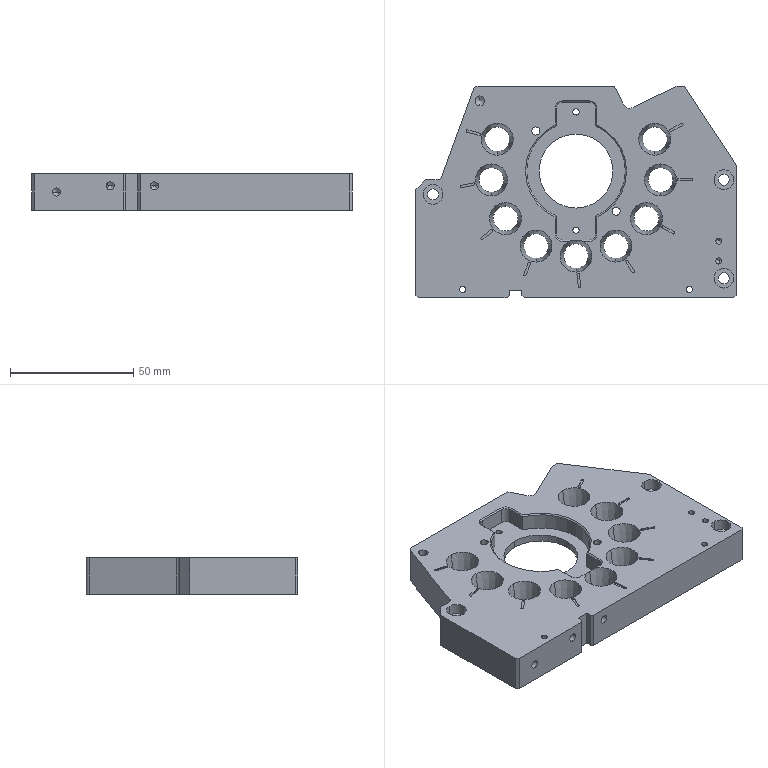NC program | NX | posted with a generic post | part box 130 x 86 x 15 mm
Whole program:
N10 G17 G21 G94 G90
(DRILLING_COPY_2 , TOOL : ZXZ)
N12 T21 M6
N14 G54
N16 G17 G0 G90 X15.25 Y-2.5 B0. C0. S3500 M3
N18 G43 Z30. H21
N20 G94 G81 G98 Z-1. F250. R3.
N22 X55. Y0.
N24 X33.25 Y-2.5
N26 G80
N28 G0 X33.25 Y-2.5 Z30.
N30 M5
(DRILLING_COPY_1_COPY_1 , TOOL : 3.3ZT)
N32 T13 M6
N34 G54
N36 G17 G0 G90 X15.25 Y-2.5 B0. C0. S2000 M3
N38 G43 Z30. H13
N40 G94 G83 G98 Z-11.091 F150. Q2. R3.
N42 X55. Y0. Z-5.991
N44 X33.25 Y-2.5 Z-11.091
N46 G80
N48 G0 X33.25 Y-2.5 Z30.
N50 M5
(ZLEVEL_PROFILE_1_COPY_COPY_1 , TOOL : D4)
N52 T17 M6
N54 G54
N56 G17 G0 G90 X24.698 Y13.381 B0. C0. S7500 M3
N58 G43 Z30. H17
N60 Z0.5
N62 G94 G1 X24.689 Y13.375 Z0.403 F1000.
N64 X24.664 Y13.354 Z0.316
N66 X24.627 Y13.318 Z0.239
N68 X24.579 Y13.264 Z0.171
N70 X24.523 Y13.192 Z0.113
N72 X24.462 Y13.098 Z0.062
N74 X24.398 Y12.981 Z0.02
N76 X24.334 Y12.84 Z-0.015
N78 X24.273 Y12.673 Z-0.043
N80 X24.217 Y12.477 Z-0.065
N82 X24.169 Y12.252 Z-0.081
N84 X24.131 Y11.996 Z-0.092
N86 X24.107 Y11.706 Z-0.098
N88 X24.098 Y11.381 Z-0.1
N90 X24.1 Y6.871 F1650.
N92 Y-7.493
N94 X24.098 Y-11.381
N96 X24.106 Y-11.461
N98 X24.127 Y-11.53
N100 X24.158 Y-11.588
N102 X24.198 Y-11.637
N104 X24.244 Y-11.676
N106 X24.292 Y-11.708
N108 X24.341 Y-11.733
N110 X24.422 Y-11.761
N112 X24.5 Y-11.77
N114 X24.578 Y-11.761
N116 X24.659 Y-11.733
N118 X24.708 Y-11.708
N120 X24.756 Y-11.676
N122 X24.802 Y-11.637
N124 X24.842 Y-11.588
N126 X24.873 Y-11.53
N128 X24.894 Y-11.461
N130 X24.902 Y-11.381
N132 Y-7.503
N134 X24.9 Y-7.485
N136 Y6.871
N138 X24.902 Y11.381
N140 X24.894 Y11.462 Z-0.101
N142 X24.873 Y11.531 Z-0.103
N144 X24.842 Y11.59 Z-0.106
N146 X24.802 Y11.639 Z-0.11
N148 X24.756 Y11.679 Z-0.115
N150 X24.708 Y11.711 Z-0.121
N152 X24.659 Y11.736 Z-0.127
N154 X24.578 Y11.765 Z-0.138
N156 X24.5 Y11.775 Z-0.15
N158 X24.422 Y11.766 Z-0.162
N160 X24.341 Y11.738 Z-0.173
N162 X24.292 Y11.714 Z-0.179
N164 X24.244 Y11.682 Z-0.185
N166 X24.198 Y11.642 Z-0.19
N168 X24.158 Y11.593 Z-0.194
N170 X24.127 Y11.535 Z-0.197
N172 X24.106 Y11.466 Z-0.199
N174 X24.098 Y11.385 Z-0.2
N176 X24.1 Y6.871
N178 Y-7.493
N180 X24.098 Y-11.385
N182 X24.106 Y-11.465
N184 X24.127 Y-11.534
N186 X24.158 Y-11.592
N188 X24.198 Y-11.641
N190 X24.244 Y-11.68
N192 X24.292 Y-11.712
N194 X24.341 Y-11.737
N196 X24.422 Y-11.765
N198 X24.5 Y-11.774
N200 X24.578 Y-11.765
N202 X24.659 Y-11.737
N204 X24.708 Y-11.712
N206 X24.756 Y-11.68
N208 X24.802 Y-11.641
N210 X24.842 Y-11.592
N212 X24.873 Y-11.534
N214 X24.894 Y-11.465
N216 X24.902 Y-11.385
N218 Y-7.503
N220 X24.9 Y-7.485
N222 Y6.871
N224 X24.902 Y11.385
N226 X24.894 Y11.466 Z-0.201
N228 X24.873 Y11.535 Z-0.203
N230 X24.842 Y11.594 Z-0.206
N232 X24.802 Y11.643 Z-0.21
N234 X24.756 Y11.683 Z-0.215
N236 X24.708 Y11.715 Z-0.221
N238 X24.659 Y11.74 Z-0.227
N240 X24.578 Y11.769 Z-0.238
N242 X24.5 Y11.779 Z-0.25
N244 X24.422 Y11.77 Z-0.262
N246 X24.341 Y11.742 Z-0.273
N248 X24.292 Y11.718 Z-0.279
N250 X24.244 Y11.686 Z-0.285
N252 X24.198 Y11.646 Z-0.29
N254 X24.159 Y11.597 Z-0.294
N256 X24.127 Y11.539 Z-0.297
N258 X24.106 Y11.47 Z-0.299
N260 X24.098 Y11.389 Z-0.3
N262 X24.1 Y6.871
N264 Y-7.493
N266 X24.098 Y-11.389
N268 X24.106 Y-11.469
N270 X24.127 Y-11.538
N272 X24.158 Y-11.596
N274 X24.198 Y-11.645
N276 X24.244 Y-11.684
N278 X24.292 Y-11.716
N280 X24.341 Y-11.741
N282 X24.422 Y-11.769
N284 X24.5 Y-11.778
N286 X24.578 Y-11.769
N288 X24.659 Y-11.741
N290 X24.708 Y-11.716
N292 X24.756 Y-11.684
N294 X24.802 Y-11.645
N296 X24.842 Y-11.596
N298 X24.873 Y-11.538
N300 X24.894 Y-11.469
N302 X24.902 Y-11.389
N304 Y-7.503
N306 X24.9 Y-7.485
N308 Y6.871
N310 X24.902 Y11.389
N312 X24.894 Y11.47 Z-0.301
N314 X24.873 Y11.539 Z-0.303
N316 X24.841 Y11.598 Z-0.306
N318 X24.802 Y11.647 Z-0.31
N320 X24.756 Y11.687 Z-0.315
N322 X24.708 Y11.719 Z-0.321
N324 X24.659 Y11.745 Z-0.327
N326 X24.578 Y11.773 Z-0.338
N328 X24.5 Y11.783 Z-0.35
N330 X24.422 Y11.774 Z-0.362
N332 X24.341 Y11.746 Z-0.373
N334 X24.292 Y11.722 Z-0.379
N336 X24.244 Y11.69 Z-0.385
N338 X24.199 Y11.65 Z-0.39
N340 X24.159 Y11.602 Z-0.394
N342 X24.127 Y11.543 Z-0.397
N344 X24.106 Y11.474 Z-0.399
N346 X24.098 Y11.393 Z-0.4
N348 X24.1 Y6.871
N350 Y-7.493
N352 X24.098 Y-11.393
N354 X24.106 Y-11.473
N356 X24.127 Y-11.542
N358 X24.158 Y-11.6
N360 X24.198 Y-11.649
N362 X24.244 Y-11.688
N364 X24.292 Y-11.72
N366 X24.341 Y-11.745
N368 X24.422 Y-11.773
N370 X24.5 Y-11.782
N372 X24.578 Y-11.773
N374 X24.659 Y-11.745
N376 X24.708 Y-11.72
N378 X24.756 Y-11.688
N380 X24.802 Y-11.649
N382 X24.841 Y-11.6
N384 X24.873 Y-11.542
N386 X24.894 Y-11.473
N388 X24.902 Y-11.393
N390 Y-7.503
N392 X24.9 Y-7.485
N394 Y6.871
N396 X24.902 Y11.393
N398 X24.894 Y11.474 Z-0.401
N400 X24.873 Y11.543 Z-0.403
N402 X24.841 Y11.602 Z-0.406
N404 X24.802 Y11.651 Z-0.41
N406 X24.756 Y11.691 Z-0.415
N408 X24.708 Y11.723 Z-0.421
N410 X24.659 Y11.749 Z-0.427
N412 X24.578 Y11.777 Z-0.438
N414 X24.5 Y11.787 Z-0.45
N416 X24.422 Y11.778 Z-0.462
N418 X24.341 Y11.75 Z-0.473
N420 X24.292 Y11.726 Z-0.479
N422 X24.244 Y11.694 Z-0.485
N424 X24.199 Y11.654 Z-0.49
N426 X24.159 Y11.606 Z-0.494
N428 X24.127 Y11.547 Z-0.497
N430 X24.106 Y11.478 Z-0.499
N432 X24.098 Y11.397 Z-0.5
N434 X24.1 Y6.871
N436 Y-7.493
N438 X24.098 Y-11.397
N440 X24.106 Y-11.478
N442 X24.127 Y-11.546
N444 X24.159 Y-11.604
N446 X24.198 Y-11.653
N448 X24.244 Y-11.692
N450 X24.292 Y-11.724
N452 X24.341 Y-11.749
N454 X24.422 Y-11.777
N456 X24.5 Y-11.787
N458 X24.578 Y-11.777
N460 X24.659 Y-11.749
N462 X24.708 Y-11.724
N464 X24.756 Y-11.692
N466 X24.802 Y-11.653
N468 X24.841 Y-11.604
N470 X24.873 Y-11.546
N472 X24.894 Y-11.478
N474 X24.902 Y-11.397
N476 Y-7.503
N478 X24.9 Y-7.485
N480 Y6.871
N482 X24.902 Y11.397
N484 X24.894 Y11.478 Z-0.501
N486 X24.873 Y11.547 Z-0.503
N488 X24.841 Y11.606 Z-0.506
N490 X24.801 Y11.655 Z-0.51
N492 X24.756 Y11.695 Z-0.515
N494 X24.708 Y11.727 Z-0.521
N496 X24.659 Y11.753 Z-0.527
N498 X24.578 Y11.782 Z-0.538
N500 X24.5 Y11.791 Z-0.55
N502 X24.422 Y11.782 Z-0.562
N504 X24.341 Y11.754 Z-0.573
N506 X24.293 Y11.73 Z-0.579
N508 X24.244 Y11.698 Z-0.585
N510 X24.199 Y11.658 Z-0.59
N512 X24.159 Y11.61 Z-0.594
N514 X24.127 Y11.551 Z-0.597
N516 X24.106 Y11.482 Z-0.599
N518 X24.098 Y11.401 Z-0.6
N520 X24.1 Y6.871
N522 Y-7.493
N524 X24.098 Y-11.402
N526 X24.106 Y-11.482
N528 X24.127 Y-11.55
N530 X24.159 Y-11.608
N532 X24.198 Y-11.657
N534 X24.244 Y-11.696
N536 X24.292 Y-11.728
N538 X24.341 Y-11.753
N540 X24.422 Y-11.781
N542 X24.5 Y-11.791
N544 X24.578 Y-11.781
N546 X24.659 Y-11.753
N548 X24.708 Y-11.728
N550 X24.756 Y-11.696
N552 X24.801 Y-11.657
N554 X24.841 Y-11.608
N556 X24.873 Y-11.55
N558 X24.894 Y-11.482
N560 X24.902 Y-11.402
N562 Y-7.503
N564 X24.9 Y-7.485
N566 Y6.871
N568 X24.902 Y11.401
N570 X24.894 Y11.482 Z-0.601
N572 X24.873 Y11.551 Z-0.603
N574 X24.841 Y11.61 Z-0.606
N576 X24.801 Y11.659 Z-0.61
N578 X24.756 Y11.699 Z-0.615
N580 X24.708 Y11.731 Z-0.621
N582 X24.659 Y11.757 Z-0.627
N584 X24.578 Y11.786 Z-0.638
N586 X24.5 Y11.796 Z-0.65
N588 X24.422 Y11.787 Z-0.662
N590 X24.341 Y11.759 Z-0.673
N592 X24.293 Y11.734 Z-0.679
N594 X24.244 Y11.702 Z-0.685
N596 X24.199 Y11.662 Z-0.69
N598 X24.159 Y11.614 Z-0.694
N600 X24.127 Y11.555 Z-0.697
N602 X24.106 Y11.486 Z-0.699
N604 X24.099 Y11.406 Z-0.7
N606 X24.1 Y6.871
N608 Y-7.493
N610 X24.099 Y-11.406
N612 X24.106 Y-11.486
N614 X24.127 Y-11.554
N616 X24.159 Y-11.612
N618 X24.198 Y-11.661
N620 X24.244 Y-11.7
N622 X24.292 Y-11.732
N624 X24.341 Y-11.757
N626 X24.422 Y-11.785
N628 X24.5 Y-11.795
N630 X24.578 Y-11.785
N632 X24.659 Y-11.757
N634 X24.708 Y-11.732
N636 X24.756 Y-11.7
N638 X24.801 Y-11.661
N640 X24.841 Y-11.612
N642 X24.873 Y-11.554
N644 X24.894 Y-11.486
N646 X24.901 Y-11.406
N648 Y-7.503
N650 X24.9 Y-7.485
N652 Y6.871
N654 X24.901 Y11.406
N656 X24.894 Y11.486 Z-0.701
N658 X24.873 Y11.555 Z-0.703
N660 X24.841 Y11.614 Z-0.706
N662 X24.801 Y11.663 Z-0.71
N664 X24.756 Y11.703 Z-0.715
N666 X24.708 Y11.736 Z-0.721
N668 X24.659 Y11.761 Z-0.727
N670 X24.578 Y11.79 Z-0.738
N672 X24.5 Y11.8 Z-0.75
N674 X24.422 Y11.791 Z-0.762
N676 X24.341 Y11.763 Z-0.773
N678 X24.293 Y11.738 Z-0.779
N680 X24.244 Y11.706 Z-0.785
N682 X24.199 Y11.666 Z-0.79
N684 X24.159 Y11.618 Z-0.794
N686 X24.127 Y11.559 Z-0.797
N688 X24.106 Y11.49 Z-0.799
N690 X24.099 Y11.41 Z-0.8
N692 X24.1 Y6.871
N694 Y-7.493
N696 X24.099 Y-11.41
N698 X24.106 Y-11.49
N700 X24.127 Y-11.558
N702 X24.159 Y-11.616
N704 X24.199 Y-11.665
N706 X24.244 Y-11.705
N708 X24.292 Y-11.736
N710 X24.341 Y-11.761
N712 X24.422 Y-11.789
N714 X24.5 Y-11.799
N716 X24.578 Y-11.789
N718 X24.659 Y-11.761
N720 X24.708 Y-11.736
N722 X24.756 Y-11.705
N724 X24.801 Y-11.665
N726 X24.841 Y-11.616
N728 X24.873 Y-11.558
N730 X24.894 Y-11.49
N732 X24.901 Y-11.41
N734 Y-7.503
N736 X24.9 Y-7.485
N738 Y6.871
N740 X24.901 Y11.41
N742 X24.894 Y11.49 Z-0.801
N744 X24.873 Y11.56 Z-0.803
N746 X24.841 Y11.618 Z-0.806
N748 X24.801 Y11.667 Z-0.81
N750 X24.756 Y11.707 Z-0.815
N752 X24.708 Y11.74 Z-0.821
N754 X24.659 Y11.765 Z-0.827
N756 X24.578 Y11.794 Z-0.838
N758 X24.5 Y11.804 Z-0.85
N760 X24.422 Y11.795 Z-0.862
N762 X24.341 Y11.767 Z-0.873
N764 X24.293 Y11.742 Z-0.879
N766 X24.244 Y11.71 Z-0.885
N768 X24.199 Y11.67 Z-0.89
N770 X24.159 Y11.622 Z-0.894
N772 X24.127 Y11.563 Z-0.897
N774 X24.106 Y11.494 Z-0.899
N776 X24.099 Y11.414 Z-0.9
N778 Y7.503
N780 X24.1 Y6.871
N782 Y-7.493
N784 X24.099 Y-11.414
N786 X24.106 Y-11.494
N788 X24.127 Y-11.562
N790 X24.159 Y-11.621
N792 X24.199 Y-11.669
N794 X24.244 Y-11.709
N796 X24.292 Y-11.74
N798 X24.341 Y-11.765
N800 X24.422 Y-11.793
N802 X24.5 Y-11.803
N804 X24.578 Y-11.793
N806 X24.659 Y-11.765
N808 X24.708 Y-11.74
N810 X24.756 Y-11.709
N812 X24.801 Y-11.669
N814 X24.841 Y-11.621
N816 X24.873 Y-11.562
N818 X24.894 Y-11.494
N820 X24.901 Y-11.414
N822 Y-7.503
N824 X24.9 Y-7.485
N826 Y6.871
N828 X24.901 Y11.414
N830 X24.894 Y11.494 Z-0.901
N832 X24.873 Y11.564 Z-0.903
N834 X24.841 Y11.622 Z-0.906
N836 X24.801 Y11.671 Z-0.91
N838 X24.756 Y11.711 Z-0.915
N840 X24.707 Y11.744 Z-0.921
N842 X24.659 Y11.769 Z-0.927
N844 X24.578 Y11.798 Z-0.938
N846 X24.5 Y11.808 Z-0.95
N848 X24.423 Y11.799 Z-0.962
N850 X24.341 Y11.771 Z-0.973
N852 X24.293 Y11.746 Z-0.979
N854 X24.244 Y11.714 Z-0.985
N856 X24.199 Y11.674 Z-0.99
N858 X24.159 Y11.626 Z-0.994
N860 X24.127 Y11.568 Z-0.997
N862 X24.106 Y11.498 Z-0.999
N864 X24.099 Y11.418 Z-1.
N866 Y7.503
N868 X24.1 Y7.214
N870 Y-7.5
N872 X24.099 Y-11.418
N874 X24.106 Y-11.498
N876 X24.127 Y-11.567
N878 X24.159 Y-11.625
N880 X24.199 Y-11.673
N882 X24.244 Y-11.713
N884 X24.292 Y-11.744
N886 X24.341 Y-11.769
N888 X24.422 Y-11.797
N890 X24.5 Y-11.807
N892 X24.578 Y-11.797
N894 X24.659 Y-11.769
N896 X24.708 Y-11.744
N898 X24.756 Y-11.713
N900 X24.801 Y-11.673
N902 X24.841 Y-11.625
N904 X24.873 Y-11.567
N906 X24.894 Y-11.498
N908 X24.901 Y-11.418
N910 Y-7.575
N912 X24.9 Y-7.5
N914 Y7.214
N916 X24.901 Y11.418
N918 X24.894 Y11.499 Z-1.001
N920 X24.873 Y11.568 Z-1.003
N922 X24.841 Y11.626 Z-1.006
N924 X24.801 Y11.675 Z-1.01
N926 X24.756 Y11.715 Z-1.015
N928 X24.707 Y11.748 Z-1.021
N930 X24.659 Y11.773 Z-1.027
N932 X24.578 Y11.802 Z-1.038
N934 X24.5 Y11.812 Z-1.05
N936 X24.423 Y11.803 Z-1.062
N938 X24.341 Y11.775 Z-1.073
N940 X24.293 Y11.75 Z-1.079
N942 X24.244 Y11.718 Z-1.085
N944 X24.199 Y11.679 Z-1.09
N946 X24.159 Y11.63 Z-1.094
N948 X24.127 Y11.572 Z-1.097
N950 X24.106 Y11.503 Z-1.099
N952 X24.099 Y11.422 Z-1.1
N954 Y7.503
N956 X24.1 Y7.214
N958 Y-7.5
N960 X24.099 Y-11.422
N962 X24.106 Y-11.502
N964 X24.127 Y-11.571
N966 X24.159 Y-11.629
N968 X24.199 Y-11.677
N970 X24.244 Y-11.717
N972 X24.292 Y-11.748
N974 X24.341 Y-11.773
N976 X24.422 Y-11.801
N978 X24.5 Y-11.811
N980 X24.578 Y-11.801
N982 X24.659 Y-11.773
N984 X24.707 Y-11.748
N986 X24.756 Y-11.717
N988 X24.801 Y-11.677
N990 X24.841 Y-11.629
N992 X24.873 Y-11.571
N994 X24.894 Y-11.502
N996 X24.901 Y-11.422
N998 Y-7.575
N1000 X24.9 Y-7.5
N1002 Y7.214
N1004 X24.901 Y11.422
N1006 X24.894 Y11.503 Z-1.101
N1008 X24.873 Y11.572 Z-1.103
N1010 X24.841 Y11.63 Z-1.106
N1012 X24.801 Y11.679 Z-1.11
N1014 X24.756 Y11.719 Z-1.115
N1016 X24.707 Y11.752 Z-1.121
N1018 X24.659 Y11.777 Z-1.127
N1020 X24.578 Y11.806 Z-1.138
N1022 X24.5 Y11.816 Z-1.15
N1024 X24.423 Y11.807 Z-1.162
N1026 X24.341 Y11.779 Z-1.173
N1028 X24.293 Y11.754 Z-1.179
N1030 X24.244 Y11.722 Z-1.185
N1032 X24.199 Y11.683 Z-1.19
N1034 X24.159 Y11.634 Z-1.194
N1036 X24.127 Y11.576 Z-1.197
N1038 X24.106 Y11.507 Z-1.199
N1040 X24.099 Y11.426 Z-1.2
N1042 Y7.503
N1044 X24.1 Y7.214
N1046 Y-7.5
N1048 X24.099 Y-11.426
N1050 X24.106 Y-11.506
N1052 X24.127 Y-11.575
N1054 X24.159 Y-11.633
N1056 X24.199 Y-11.681
N1058 X24.244 Y-11.721
N1060 X24.292 Y-11.752
N1062 X24.341 Y-11.777
N1064 X24.422 Y-11.805
N1066 X24.5 Y-11.815
N1068 X24.578 Y-11.805
N1070 X24.659 Y-11.777
N1072 X24.707 Y-11.752
N1074 X24.756 Y-11.721
N1076 X24.801 Y-11.681
N1078 X24.841 Y-11.633
N1080 X24.873 Y-11.575
N1082 X24.894 Y-11.506
N1084 X24.901 Y-11.426
N1086 Y-7.575
N1088 X24.9 Y-7.5
N1090 Y7.214
N1092 X24.901 Y11.426
N1094 X24.894 Y11.507 Z-1.201
N1096 X24.873 Y11.576 Z-1.203
N1098 X24.841 Y11.634 Z-1.206
N1100 X24.801 Y11.683 Z-1.21
N1102 X24.756 Y11.724 Z-1.215
N1104 X24.707 Y11.756 Z-1.221
N1106 X24.659 Y11.781 Z-1.227
N1108 X24.578 Y11.81 Z-1.238
N1110 X24.5 Y11.82 Z-1.25
N1112 X24.423 Y11.811 Z-1.262
N1114 X24.341 Y11.783 Z-1.273
N1116 X24.293 Y11.758 Z-1.279
N1118 X24.244 Y11.726 Z-1.285
N1120 X24.199 Y11.687 Z-1.29
N1122 X24.159 Y11.638 Z-1.294
N1124 X24.127 Y11.58 Z-1.297
N1126 X24.106 Y11.511 Z-1.299
N1128 X24.099 Y11.43 Z-1.3
N1130 Y7.503
N1132 X24.1 Y7.214
N1134 Y-7.5
N1136 X24.099 Y-11.43
N1138 X24.106 Y-11.51
N1140 X24.127 Y-11.579
N1142 X24.159 Y-11.637
N1144 X24.199 Y-11.685
N1146 X24.244 Y-11.725
N1148 X24.293 Y-11.757
N1150 X24.341 Y-11.781
N1152 X24.422 Y-11.809
N1154 X24.5 Y-11.819
N1156 X24.578 Y-11.809
N1158 X24.659 Y-11.781
N1160 X24.707 Y-11.757
N1162 X24.756 Y-11.725
N1164 X24.801 Y-11.685
N1166 X24.841 Y-11.637
N1168 X24.873 Y-11.579
N1170 X24.894 Y-11.51
N1172 X24.901 Y-11.43
N1174 Y-7.575
N1176 X24.9 Y-7.5
N1178 Y7.214
N1180 X24.901 Y11.43
N1182 X24.894 Y11.511 Z-1.301
N1184 X24.873 Y11.58 Z-1.303
N1186 X24.841 Y11.639 Z-1.306
N1188 X24.801 Y11.687 Z-1.31
N1190 X24.756 Y11.728 Z-1.315
N1192 X24.707 Y11.76 Z-1.321
N1194 X24.659 Y11.785 Z-1.327
N1196 X24.578 Y11.814 Z-1.338
N1198 X24.5 Y11.824 Z-1.35
N1200 X24.423 Y11.815 Z-1.362
N1202 X24.342 Y11.787 Z-1.373
N1204 X24.293 Y11.762 Z-1.379
N1206 X24.244 Y11.73 Z-1.385
N1208 X24.199 Y11.691 Z-1.39
N1210 X24.159 Y11.642 Z-1.394
N1212 X24.128 Y11.584 Z-1.397
N1214 X24.107 Y11.515 Z-1.399
N1216 X24.099 Y11.434 Z-1.4
N1218 Y7.503
N1220 X24.1 Y7.214
N1222 Y-7.5
N1224 X24.099 Y-11.434
N1226 X24.107 Y-11.514
N1228 X24.127 Y-11.583
N1230 X24.159 Y-11.641
N1232 X24.199 Y-11.689
N1234 X24.244 Y-11.729
N1236 X24.293 Y-11.761
N1238 X24.341 Y-11.785
N1240 X24.422 Y-11.813
N1242 X24.5 Y-11.823
N1244 X24.578 Y-11.813
N1246 X24.659 Y-11.785
N1248 X24.707 Y-11.761
N1250 X24.756 Y-11.729
N1252 X24.801 Y-11.689
N1254 X24.841 Y-11.641
N1256 X24.873 Y-11.583
N1258 X24.893 Y-11.514
N1260 X24.901 Y-11.434
N1262 Y-7.575
N1264 X24.9 Y-7.5
N1266 Y7.214
N1268 X24.901 Y11.434
N1270 X24.893 Y11.515 Z-1.401
N1272 X24.873 Y11.584 Z-1.403
N1274 X24.841 Y11.643 Z-1.406
N1276 X24.801 Y11.692 Z-1.41
N1278 X24.756 Y11.732 Z-1.415
N1280 X24.707 Y11.764 Z-1.421
N1282 X24.659 Y11.789 Z-1.427
N1284 X24.578 Y11.818 Z-1.438
N1286 X24.5 Y11.828 Z-1.45
N1288 X24.423 Y11.819 Z-1.462
N1290 X24.342 Y11.791 Z-1.473
N1292 X24.293 Y11.766 Z-1.479
N1294 X24.245 Y11.734 Z-1.485
N1296 X24.199 Y11.695 Z-1.49
N1298 X24.159 Y11.646 Z-1.494
N1300 X24.128 Y11.588 Z-1.497
N1302 X24.107 Y11.519 Z-1.499
N1304 X24.099 Y11.438 Z-1.5
N1306 Y7.503
N1308 X24.1 Y7.214
N1310 Y-7.5
N1312 X24.099 Y-11.438
N1314 X24.107 Y-11.518
N1316 X24.127 Y-11.587
N1318 X24.159 Y-11.645
N1320 X24.199 Y-11.693
N1322 X24.244 Y-11.733
N1324 X24.293 Y-11.765
N1326 X24.341 Y-11.789
N1328 X24.422 Y-11.817
N1330 X24.5 Y-11.827
N1332 X24.578 Y-11.817
N1334 X24.659 Y-11.789
N1336 X24.707 Y-11.765
N1338 X24.756 Y-11.733
N1340 X24.801 Y-11.693
N1342 X24.841 Y-11.645
N1344 X24.872 Y-11.587
N1346 X24.893 Y-11.518
N1348 X24.901 Y-11.438
N1350 Y-7.575
N1352 X24.9 Y-7.5
N1354 Y7.214
N1356 X24.901 Y11.438
N1358 X24.893 Y11.519 Z-1.501
N1360 X24.872 Y11.588 Z-1.503
N1362 X24.841 Y11.647 Z-1.506
N1364 X24.801 Y11.696 Z-1.51
N1366 X24.756 Y11.736 Z-1.515
N1368 X24.707 Y11.768 Z-1.521
N1370 X24.659 Y11.793 Z-1.527
N1372 X24.578 Y11.822 Z-1.538
N1374 X24.5 Y11.832 Z-1.55
N1376 X24.423 Y11.823 Z-1.562
N1378 X24.342 Y11.795 Z-1.573
N1380 X24.293 Y11.77 Z-1.579
N1382 X24.245 Y11.739 Z-1.585
N1384 X24.199 Y11.699 Z-1.59
N1386 X24.159 Y11.65 Z-1.594
N1388 X24.128 Y11.592 Z-1.597
N1390 X24.107 Y11.523 Z-1.599
N1392 X24.099 Y11.442 Z-1.6
N1394 Y7.503
N1396 X24.1 Y7.214
N1398 Y-7.5
N1400 X24.099 Y-11.443
N1402 X24.107 Y-11.522
N1404 X24.128 Y-11.591
N1406 X24.159 Y-11.649
N1408 X24.199 Y-11.697
N1410 X24.244 Y-11.737
N1412 X24.293 Y-11.769
N1414 X24.341 Y-11.793
N1416 X24.422 Y-11.822
N1418 X24.5 Y-11.831
N1420 X24.578 Y-11.822
N1422 X24.659 Y-11.793
N1424 X24.707 Y-11.769
N1426 X24.756 Y-11.737
N1428 X24.801 Y-11.697
N1430 X24.841 Y-11.649
N1432 X24.872 Y-11.591
N1434 X24.893 Y-11.522
N1436 X24.901 Y-11.443
N1438 Y-7.575
N1440 X24.9 Y-7.5
N1442 Y7.214
N1444 X24.901 Y11.442
N1446 X24.893 Y11.523 Z-1.601
N1448 X24.872 Y11.592 Z-1.603
N1450 X24.841 Y11.651 Z-1.606
N1452 X24.801 Y11.7 Z-1.61
N1454 X24.756 Y11.74 Z-1.615
N1456 X24.707 Y11.772 Z-1.621
N1458 X24.659 Y11.797 Z-1.627
N1460 X24.578 Y11.826 Z-1.638
N1462 X24.5 Y11.836 Z-1.65
N1464 X24.423 Y11.827 Z-1.662
N1466 X24.342 Y11.799 Z-1.673
N1468 X24.293 Y11.774 Z-1.679
N1470 X24.245 Y11.743 Z-1.685
N1472 X24.199 Y11.703 Z-1.69
N1474 X24.159 Y11.654 Z-1.694
N1476 X24.128 Y11.596 Z-1.697
N1478 X24.107 Y11.527 Z-1.699
N1480 X24.099 Y11.447 Z-1.7
N1482 Y7.503
N1484 X24.1 Y7.214
N1486 Y-7.5
N1488 X24.099 Y-11.447
N1490 X24.107 Y-11.527
N1492 X24.128 Y-11.595
N1494 X24.159 Y-11.653
N1496 X24.199 Y-11.701
N1498 X24.244 Y-11.741
N1500 X24.293 Y-11.773
N1502 X24.341 Y-11.797
N1504 X24.422 Y-11.826
N1506 X24.5 Y-11.835
N1508 X24.577 Y-11.826
N1510 X24.659 Y-11.797
N1512 X24.707 Y-11.773
N1514 X24.755 Y-11.741
N1516 X24.801 Y-11.701
N1518 X24.841 Y-11.653
N1520 X24.872 Y-11.595
N1522 X24.893 Y-11.527
N1524 X24.901 Y-11.447
N1526 X24.902 Y-7.593
N1528 X24.9 Y-7.5
N1530 Y7.214
N1532 X24.901 Y11.447
N1534 X24.893 Y11.527 Z-1.701
N1536 X24.872 Y11.596 Z-1.703
N1538 X24.841 Y11.655 Z-1.706
N1540 X24.801 Y11.704 Z-1.71
N1542 X24.755 Y11.744 Z-1.715
N1544 X24.707 Y11.776 Z-1.721
N1546 X24.659 Y11.801 Z-1.727
N1548 X24.578 Y11.83 Z-1.738
N1550 X24.5 Y11.84 Z-1.75
N1552 X24.423 Y11.831 Z-1.762
N1554 X24.342 Y11.803 Z-1.773
N1556 X24.293 Y11.778 Z-1.779
N1558 X24.245 Y11.747 Z-1.785
N1560 X24.199 Y11.707 Z-1.79
N1562 X24.159 Y11.658 Z-1.794
N1564 X24.128 Y11.6 Z-1.797
N1566 X24.107 Y11.531 Z-1.799
N1568 X24.099 Y11.451 Z-1.8
N1570 Y7.503
N1572 X24.1 Y7.214
N1574 Y-7.5
N1576 X24.099 Y-11.451
N1578 X24.107 Y-11.531
N1580 X24.128 Y-11.599
N1582 X24.159 Y-11.657
N1584 X24.199 Y-11.705
N1586 X24.244 Y-11.745
N1588 X24.293 Y-11.777
N1590 X24.341 Y-11.801
N1592 X24.422 Y-11.83
N1594 X24.5 Y-11.839
N1596 X24.577 Y-11.83
N1598 X24.659 Y-11.801
N1600 X24.707 Y-11.777
N1602 X24.755 Y-11.745
N1604 X24.801 Y-11.705
N1606 X24.841 Y-11.657
N1608 X24.872 Y-11.599
N1610 X24.893 Y-11.531
N1612 X24.901 Y-11.451
N1614 X24.902 Y-7.593
N1616 X24.9 Y-7.5
N1618 Y7.214
N1620 X24.901 Y11.451
N1622 X24.893 Y11.531 Z-1.801
N1624 X24.872 Y11.6 Z-1.803
N1626 X24.841 Y11.659 Z-1.806
N1628 X24.801 Y11.708 Z-1.81
N1630 X24.755 Y11.748 Z-1.815
N1632 X24.707 Y11.78 Z-1.821
N1634 X24.658 Y11.805 Z-1.827
N1636 X24.578 Y11.834 Z-1.838
N1638 X24.5 Y11.844 Z-1.85
N1640 X24.423 Y11.835 Z-1.862
N1642 X24.342 Y11.807 Z-1.873
N1644 X24.293 Y11.782 Z-1.879
N1646 X24.245 Y11.751 Z-1.885
N1648 X24.199 Y11.711 Z-1.89
N1650 X24.159 Y11.662 Z-1.894
N1652 X24.128 Y11.604 Z-1.897
N1654 X24.107 Y11.535 Z-1.899
N1656 X24.099 Y11.455 Z-1.9
N1658 X24.1 Y7.214
N1660 Y-7.5
N1662 X24.099 Y-11.455
N1664 X24.107 Y-11.535
N1666 X24.128 Y-11.603
N1668 X24.159 Y-11.661
N1670 X24.199 Y-11.71
N1672 X24.244 Y-11.749
N1674 X24.293 Y-11.781
N1676 X24.341 Y-11.805
N1678 X24.422 Y-11.834
N1680 X24.5 Y-11.843
N1682 X24.578 Y-11.834
N1684 X24.659 Y-11.805
N1686 X24.707 Y-11.781
N1688 X24.756 Y-11.749
N1690 X24.801 Y-11.71
N1692 X24.841 Y-11.661
N1694 X24.872 Y-11.603
N1696 X24.893 Y-11.535
N1698 X24.901 Y-11.455
N1700 X24.9 Y-7.5
N1702 Y7.214
N1704 X24.901 Y11.455
N1706 X24.893 Y11.535 Z-1.901
N1708 X24.872 Y11.604 Z-1.903
N1710 X24.841 Y11.663 Z-1.906
N1712 X24.801 Y11.712 Z-1.91
N1714 X24.755 Y11.752 Z-1.915
N1716 X24.707 Y11.784 Z-1.921
N1718 X24.658 Y11.809 Z-1.927
N1720 X24.577 Y11.838 Z-1.938
N1722 X24.5 Y11.848 Z-1.95
N1724 X24.423 Y11.839 Z-1.962
N1726 X24.342 Y11.811 Z-1.973
N1728 X24.293 Y11.786 Z-1.979
N1730 X24.245 Y11.755 Z-1.985
N1732 X24.199 Y11.715 Z-1.99
N1734 X24.16 Y11.667 Z-1.994
N1736 X24.128 Y11.608 Z-1.997
N1738 X24.107 Y11.539 Z-1.999
N1740 X24.099 Y11.459 Z-2.
N1742 X24.1 Y7.214
N1744 Y-7.5
N1746 X24.099 Y-11.459
N1748 X24.107 Y-11.539
N1750 X24.128 Y-11.607
N1752 X24.159 Y-11.665
N1754 X24.199 Y-11.714
N1756 X24.245 Y-11.753
N1758 X24.293 Y-11.785
N1760 X24.341 Y-11.809
N1762 X24.422 Y-11.838
N1764 X24.5 Y-11.847
N1766 X24.578 Y-11.838
N1768 X24.659 Y-11.809
N1770 X24.707 Y-11.785
N1772 X24.755 Y-11.753
N1774 X24.801 Y-11.714
N1776 X24.841 Y-11.665
N1778 X24.872 Y-11.607
N1780 X24.893 Y-11.539
N1782 X24.901 Y-11.459
N1784 X24.9 Y-7.5
N1786 Y7.214
N1788 X24.901 Y11.459
N1790 X24.893 Y11.539 Z-2.001
N1792 X24.872 Y11.608 Z-2.003
N1794 X24.84 Y11.667 Z-2.006
N1796 X24.801 Y11.716 Z-2.01
N1798 X24.755 Y11.756 Z-2.015
N1800 X24.707 Y11.788 Z-2.021
N1802 X24.658 Y11.813 Z-2.027
N1804 X24.577 Y11.842 Z-2.038
N1806 X24.5 Y11.852 Z-2.05
N1808 X24.423 Y11.843 Z-2.062
N1810 X24.342 Y11.815 Z-2.073
N1812 X24.293 Y11.79 Z-2.079
N1814 X24.245 Y11.759 Z-2.085
N1816 X24.199 Y11.719 Z-2.09
N1818 X24.16 Y11.671 Z-2.094
N1820 X24.128 Y11.612 Z-2.097
N1822 X24.107 Y11.543 Z-2.099
N1824 X24.099 Y11.463 Z-2.1
N1826 X24.1 Y7.214
N1828 Y-7.5
N1830 X24.099 Y-11.463
N1832 X24.107 Y-11.543
N1834 X24.128 Y-11.611
N1836 X24.159 Y-11.669
N1838 X24.199 Y-11.718
N1840 X24.245 Y-11.757
N1842 X24.293 Y-11.789
N1844 X24.341 Y-11.814
N1846 X24.422 Y-11.842
N1848 X24.5 Y-11.851
N1850 X24.578 Y-11.842
N1852 X24.659 Y-11.814
N1854 X24.707 Y-11.789
N1856 X24.755 Y-11.757
N1858 X24.801 Y-11.718
N1860 X24.841 Y-11.669
N1862 X24.872 Y-11.611
N1864 X24.893 Y-11.543
N1866 X24.901 Y-11.463
N1868 X24.9 Y-7.5
N1870 Y7.214
N1872 X24.901 Y11.463
N1874 X24.893 Y11.543 Z-2.101
N1876 X24.872 Y11.613 Z-2.103
N1878 X24.84 Y11.671 Z-2.106
N1880 X24.801 Y11.72 Z-2.11
N1882 X24.755 Y11.76 Z-2.115
N1884 X24.707 Y11.792 Z-2.121
N1886 X24.658 Y11.817 Z-2.127
N1888 X24.577 Y11.846 Z-2.138
N1890 X24.5 Y11.856 Z-2.15
N1892 X24.423 Y11.847 Z-2.162
N1894 X24.342 Y11.819 Z-2.173
N1896 X24.293 Y11.794 Z-2.179
N1898 X24.245 Y11.763 Z-2.185
N1900 X24.199 Y11.723 Z-2.19
N1902 X24.16 Y11.675 Z-2.194
N1904 X24.128 Y11.616 Z-2.197
N1906 X24.107 Y11.547 Z-2.199
N1908 X24.1 Y11.467 Z-2.2
N1910 Y7.214
N1912 Y-7.5
N1914 Y-11.467
N1916 X24.107 Y-11.547
N1918 X24.128 Y-11.615
N1920 X24.16 Y-11.673
N1922 X24.199 Y-11.722
N1924 X24.245 Y-11.761
N1926 X24.293 Y-11.793
N1928 X24.341 Y-11.818
N1930 X24.422 Y-11.846
N1932 X24.5 Y-11.855
N1934 X24.578 Y-11.846
N1936 X24.659 Y-11.818
N1938 X24.707 Y-11.793
N1940 X24.755 Y-11.761
N1942 X24.801 Y-11.722
N1944 X24.84 Y-11.673
N1946 X24.872 Y-11.615
N1948 X24.893 Y-11.547
N1950 X24.9 Y-11.467
N1952 Y-7.5
N1954 Y7.214
N1956 Y11.467
N1958 X24.893 Y11.548 Z-2.201
N1960 X24.872 Y11.617 Z-2.203
N1962 X24.84 Y11.675 Z-2.206
N1964 X24.801 Y11.724 Z-2.21
N1966 X24.755 Y11.764 Z-2.215
N1968 X24.707 Y11.796 Z-2.221
N1970 X24.658 Y11.821 Z-2.227
N1972 X24.577 Y11.85 Z-2.238
N1974 X24.5 Y11.86 Z-2.25
N1976 X24.423 Y11.851 Z-2.262
N1978 X24.342 Y11.823 Z-2.273
N1980 X24.293 Y11.799 Z-2.279
N1982 X24.245 Y11.767 Z-2.285
N1984 X24.199 Y11.727 Z-2.29
N1986 X24.16 Y11.679 Z-2.294
N1988 X24.128 Y11.62 Z-2.297
N1990 X24.107 Y11.552 Z-2.299
N1992 X24.1 Y11.471 Z-2.3
N1994 Y7.214
N1996 Y-7.5
N1998 Y-11.471
N2000 X24.107 Y-11.551
N2002 X24.128 Y-11.62
N2004 X24.16 Y-11.677
N2006 X24.199 Y-11.726
N2008 X24.245 Y-11.765
N2010 X24.293 Y-11.797
N2012 X24.341 Y-11.822
N2014 X24.422 Y-11.85
N2016 X24.5 Y-11.859
N2018 X24.578 Y-11.85
N2020 X24.659 Y-11.822
N2022 X24.707 Y-11.797
N2024 X24.755 Y-11.765
N2026 X24.801 Y-11.726
N2028 X24.84 Y-11.677
N2030 X24.872 Y-11.62
N2032 X24.893 Y-11.551
N2034 X24.9 Y-11.471
N2036 Y-7.5
N2038 Y7.214
N2040 Y11.471
N2042 X24.893 Y11.552 Z-2.301
N2044 X24.872 Y11.621 Z-2.303
N2046 X24.84 Y11.679 Z-2.306
N2048 X24.801 Y11.728 Z-2.31
N2050 X24.755 Y11.768 Z-2.315
N2052 X24.707 Y11.8 Z-2.321
N2054 X24.658 Y11.825 Z-2.327
N2056 X24.577 Y11.854 Z-2.338
N2058 X24.5 Y11.864 Z-2.35
N2060 X24.423 Y11.855 Z-2.362
N2062 X24.342 Y11.827 Z-2.373
N2064 X24.293 Y11.803 Z-2.379
N2066 X24.245 Y11.771 Z-2.385
N2068 X24.2 Y11.731 Z-2.39
N2070 X24.16 Y11.683 Z-2.394
N2072 X24.128 Y11.625 Z-2.397
N2074 X24.107 Y11.556 Z-2.399
N2076 X24.1 Y11.475 Z-2.4
N2078 Y7.214
N2080 Y-7.5
N2082 Y-11.475
N2084 X24.107 Y-11.555
N2086 X24.128 Y-11.624
N2088 X24.16 Y-11.682
N2090 X24.199 Y-11.73
N2092 X24.245 Y-11.769
N2094 X24.293 Y-11.801
N2096 X24.342 Y-11.826
N2098 X24.422 Y-11.854
N2100 X24.5 Y-11.863
N2102 X24.578 Y-11.854
N2104 X24.658 Y-11.826
N2106 X24.707 Y-11.801
N2108 X24.755 Y-11.769
N2110 X24.801 Y-11.73
N2112 X24.84 Y-11.682
N2114 X24.872 Y-11.624
N2116 X24.893 Y-11.555
N2118 X24.9 Y-11.475
N2120 Y-7.5
N2122 Y7.214
N2124 Y11.475
N2126 X24.893 Y11.556 Z-2.401
N2128 X24.872 Y11.625 Z-2.403
N2130 X24.84 Y11.683 Z-2.406
N2132 X24.8 Y11.732 Z-2.41
N2134 X24.755 Y11.772 Z-2.415
N2136 X24.707 Y11.804 Z-2.421
N2138 X24.658 Y11.829 Z-2.427
N2140 X24.577 Y11.858 Z-2.438
N2142 X24.5 Y11.868 Z-2.45
N2144 X24.423 Y11.859 Z-2.462
N2146 X24.342 Y11.831 Z-2.473
N2148 X24.293 Y11.807 Z-2.479
N2150 X24.245 Y11.775 Z-2.485
N2152 X24.2 Y11.735 Z-2.49
N2154 X24.16 Y11.687 Z-2.494
N2156 X24.128 Y11.629 Z-2.497
N2158 X24.107 Y11.56 Z-2.499
N2160 X24.1 Y11.479 Z-2.5
N2162 Y7.214
N2164 Y-7.5
N2166 Y-11.479
N2168 X24.107 Y-11.559
N2170 X24.128 Y-11.628
N2172 X24.16 Y-11.686
N2174 X24.199 Y-11.734
N2176 X24.245 Y-11.773
N2178 X24.293 Y-11.805
N2180 X24.342 Y-11.83
N2182 X24.422 Y-11.858
N2184 X24.5 Y-11.867
N2186 X24.578 Y-11.858
N2188 X24.658 Y-11.83
N2190 X24.707 Y-11.805
N2192 X24.755 Y-11.773
N2194 X24.801 Y-11.734
N2196 X24.84 Y-11.686
N2198 X24.872 Y-11.628
N2200 X24.893 Y-11.559
N2202 X24.9 Y-11.479
N2204 Y-7.5
N2206 Y7.214
N2208 Y11.479
N2210 X24.893 Y11.56 Z-2.501
N2212 X24.872 Y11.629 Z-2.503
N2214 X24.84 Y11.687 Z-2.506
N2216 X24.8 Y11.736 Z-2.51
N2218 X24.755 Y11.776 Z-2.515
N2220 X24.707 Y11.808 Z-2.521
N2222 X24.658 Y11.833 Z-2.527
N2224 X24.577 Y11.862 Z-2.538
N2226 X24.5 Y11.872 Z-2.55
N2228 X24.423 Y11.863 Z-2.562
N2230 X24.342 Y11.835 Z-2.573
N2232 X24.293 Y11.811 Z-2.579
N2234 X24.245 Y11.779 Z-2.585
N2236 X24.2 Y11.739 Z-2.59
N2238 X24.16 Y11.691 Z-2.594
N2240 X24.128 Y11.633 Z-2.597
N2242 X24.107 Y11.564 Z-2.599
N2244 X24.1 Y11.483 Z-2.6
N2246 Y7.214
N2248 Y-7.5
N2250 Y-11.484
N2252 X24.107 Y-11.563
N2254 X24.128 Y-11.632
N2256 X24.16 Y-11.69
N2258 X24.2 Y-11.738
N2260 X24.245 Y-11.777
N2262 X24.293 Y-11.809
N2264 X24.342 Y-11.834
N2266 X24.423 Y-11.862
N2268 X24.5 Y-11.871
N2270 X24.577 Y-11.862
N2272 X24.658 Y-11.834
N2274 X24.707 Y-11.809
N2276 X24.755 Y-11.777
N2278 X24.8 Y-11.738
N2280 X24.84 Y-11.69
N2282 X24.872 Y-11.632
N2284 X24.893 Y-11.563
N2286 X24.9 Y-11.484
N2288 Y-7.5
N2290 Y7.214
N2292 Y11.483
N2294 X24.893 Y11.564 Z-2.601
N2296 X24.872 Y11.633 Z-2.603
N2298 X24.84 Y11.691 Z-2.606
N2300 X24.8 Y11.74 Z-2.61
N2302 X24.755 Y11.78 Z-2.615
N2304 X24.707 Y11.812 Z-2.621
N2306 X24.658 Y11.837 Z-2.627
N2308 X24.577 Y11.866 Z-2.638
N2310 X24.5 Y11.876 Z-2.65
N2312 X24.423 Y11.867 Z-2.662
N2314 X24.342 Y11.839 Z-2.673
N2316 X24.293 Y11.815 Z-2.679
N2318 X24.245 Y11.783 Z-2.685
N2320 X24.2 Y11.743 Z-2.69
N2322 X24.16 Y11.695 Z-2.694
N2324 X24.128 Y11.637 Z-2.697
N2326 X24.107 Y11.568 Z-2.699
N2328 X24.1 Y11.488 Z-2.7
N2330 Y7.214
N2332 Y-7.5
N2334 Y-11.488
N2336 X24.107 Y-11.567
N2338 X24.128 Y-11.636
N2340 X24.16 Y-11.694
N2342 X24.2 Y-11.742
N2344 X24.245 Y-11.781
N2346 X24.293 Y-11.813
N2348 X24.342 Y-11.838
N2350 X24.423 Y-11.866
N2352 X24.5 Y-11.875
N2354 X24.577 Y-11.866
N2356 X24.658 Y-11.838
N2358 X24.707 Y-11.813
N2360 X24.755 Y-11.781
N2362 X24.8 Y-11.742
N2364 X24.84 Y-11.694
N2366 X24.872 Y-11.636
N2368 X24.893 Y-11.567
N2370 X24.9 Y-11.488
N2372 Y-7.5
N2374 Y7.214
N2376 Y11.488
N2378 X24.893 Y11.568 Z-2.701
N2380 X24.872 Y11.637 Z-2.703
N2382 X24.84 Y11.695 Z-2.706
N2384 X24.8 Y11.744 Z-2.71
N2386 X24.755 Y11.784 Z-2.715
N2388 X24.707 Y11.816 Z-2.721
N2390 X24.658 Y11.841 Z-2.727
N2392 X24.577 Y11.87 Z-2.738
N2394 X24.5 Y11.88 Z-2.75
N2396 X24.423 Y11.871 Z-2.762
N2398 X24.342 Y11.843 Z-2.773
N2400 X24.293 Y11.819 Z-2.779
N2402 X24.245 Y11.787 Z-2.785
N2404 X24.2 Y11.747 Z-2.79
N2406 X24.16 Y11.699 Z-2.794
N2408 X24.128 Y11.641 Z-2.797
N2410 X24.107 Y11.572 Z-2.799
N2412 X24.1 Y11.492 Z-2.8
N2414 Y7.214
N2416 Y-7.5
N2418 Y-11.492
N2420 X24.107 Y-11.572
N2422 X24.128 Y-11.64
N2424 X24.16 Y-11.698
N2426 X24.2 Y-11.746
N2428 X24.245 Y-11.786
N2430 X24.293 Y-11.817
N2432 X24.342 Y-11.842
N2434 X24.423 Y-11.87
N2436 X24.5 Y-11.879
N2438 X24.577 Y-11.87
N2440 X24.658 Y-11.842
N2442 X24.707 Y-11.817
N2444 X24.755 Y-11.786
N2446 X24.8 Y-11.746
N2448 X24.84 Y-11.698
N2450 X24.872 Y-11.64
N2452 X24.893 Y-11.572
N2454 X24.9 Y-11.492
N2456 Y-7.5
N2458 Y7.214
N2460 Y11.492
N2462 X24.893 Y11.572 Z-2.801
N2464 X24.872 Y11.641 Z-2.803
N2466 X24.84 Y11.699 Z-2.806
N2468 X24.8 Y11.748 Z-2.81
N2470 X24.755 Y11.788 Z-2.815
N2472 X24.707 Y11.82 Z-2.821
N2474 X24.658 Y11.845 Z-2.827
N2476 X24.577 Y11.874 Z-2.838
N2478 X24.5 Y11.884 Z-2.85
N2480 X24.423 Y11.875 Z-2.862
N2482 X24.342 Y11.847 Z-2.873
N2484 X24.293 Y11.823 Z-2.879
N2486 X24.245 Y11.791 Z-2.885
N2488 X24.2 Y11.752 Z-2.89
N2490 X24.16 Y11.703 Z-2.894
N2492 X24.128 Y11.645 Z-2.897
N2494 X24.108 Y11.576 Z-2.899
N2496 X24.1 Y11.496 Z-2.9
N2498 Y7.214
N2500 Y-7.5
N2502 Y-11.496
N2504 X24.108 Y-11.576
N2506 X24.128 Y-11.644
N2508 X24.16 Y-11.702
N2510 X24.2 Y-11.75
N2512 X24.245 Y-11.79
N2514 X24.293 Y-11.821
N2516 X24.342 Y-11.846
N2518 X24.423 Y-11.874
N2520 X24.5 Y-11.883
N2522 X24.577 Y-11.874
N2524 X24.658 Y-11.846
N2526 X24.707 Y-11.821
N2528 X24.755 Y-11.79
N2530 X24.8 Y-11.75
N2532 X24.84 Y-11.702
N2534 X24.872 Y-11.644
N2536 X24.892 Y-11.576
N2538 X24.9 Y-11.496
N2540 Y-7.5
N2542 Y7.214
N2544 Y11.496
N2546 X24.892 Y11.576 Z-2.901
N2548 X24.872 Y11.645 Z-2.903
N2550 X24.84 Y11.704 Z-2.906
N2552 X24.8 Y11.752 Z-2.91
N2554 X24.755 Y11.792 Z-2.915
N2556 X24.707 Y11.824 Z-2.921
N2558 X24.658 Y11.85 Z-2.927
N2560 X24.577 Y11.878 Z-2.938
N2562 X24.5 Y11.888 Z-2.95
N2564 X24.423 Y11.879 Z-2.962
N2566 X24.342 Y11.851 Z-2.973
N2568 X24.293 Y11.827 Z-2.979
N2570 X24.245 Y11.795 Z-2.985
N2572 X24.2 Y11.755 Z-2.99
N2574 X24.16 Y11.707 Z-2.994
N2576 X24.128 Y11.649 Z-2.997
N2578 X24.108 Y11.58 Z-2.999
N2580 X24.1 Y11.5 Z-3.
N2582 Y7.214
N2584 Y-7.5
N2586 Y-11.5
N2588 X24.108 Y-11.58
N2590 X24.128 Y-11.648
N2592 X24.16 Y-11.706
N2594 X24.2 Y-11.754
N2596 X24.245 Y-11.794
N2598 X24.293 Y-11.825
N2600 X24.342 Y-11.85
N2602 X24.423 Y-11.878
N2604 X24.5 Y-11.887
N2606 X24.577 Y-11.878
N2608 X24.658 Y-11.85
N2610 X24.707 Y-11.825
N2612 X24.755 Y-11.794
N2614 X24.8 Y-11.754
N2616 X24.84 Y-11.706
N2618 X24.872 Y-11.648
N2620 X24.892 Y-11.58
N2622 X24.9 Y-11.5
N2624 Y-7.5
N2626 Y7.214
N2628 Y11.5
N2630 X24.891 Y11.824 Z-2.998
N2632 X24.867 Y12.114 Z-2.992
N2634 X24.829 Y12.371 Z-2.981
N2636 X24.781 Y12.596 Z-2.965
N2638 X24.725 Y12.791 Z-2.943
N2640 X24.664 Y12.959 Z-2.915
N2642 X24.6 Y13.1 Z-2.88
N2644 X24.536 Y13.216 Z-2.838
N2646 X24.475 Y13.31 Z-2.787
N2648 X24.419 Y13.383 Z-2.729
N2650 X24.371 Y13.437 Z-2.661
N2652 X24.333 Y13.473 Z-2.584
N2654 X24.309 Y13.493 Z-2.497
N2656 X24.3 Y13.5 Z-2.4
N2658 G0 Z30.
N2660 M5
(PLANAR_MILL_COPY_1_COPY_COPY_1 , TOOL : D6A45)
N2662 T01 M6
N2664 G54
N2666 G17 G0 G90 X24.2 Y8.973 B0. C0. S7500 M3
N2668 G43 Z30. H1
N2670 Z0.
N2672 G94 G1 Z-2. F1250.
N2674 X23.357 Y8.266
N2676 G3 X23. Y7.5 R1.
N2678 G1 Y-7.5
N2680 G3 X23.357 Y-8.266 R1.
N2682 G1 X24.2 Y-8.973
N2684 Z0.
N2686 G0 Z30.
N2688 X24.8
N2690 Z0.
N2692 G1 Z-2.
N2694 X25.643 Y-8.266
N2696 G3 X26. Y-7.5 R1.
N2698 G1 Y7.5
N2700 G3 X25.643 Y8.266 R1.
N2702 G1 X24.8 Y8.973
N2704 Z0.
N2706 G0 Z30.
(PLANAR_MILL_COPY_1_COPY_COPY_1_COPY , TOOL : D6A45)
N2708 X55.95 Y0.145
N2710 Z1.
N2712 G1 Y0.241 Z0.974
N2714 X55.693 Y0.693 Z0.835
N2716 X55.241 Y0.95 Z0.696
N2718 X54.759 Z0.567
N2720 X54.307 Y0.693 Z0.427
N2722 X54.05 Y0.241 Z0.288
N2724 Y-0.241 Z0.159
N2726 X54.307 Y-0.693 Z0.019
N2728 X54.759 Y-0.95 Z-0.12
N2730 X55.241 Z-0.249
N2732 X55.693 Y-0.693 Z-0.388
N2734 X55.95 Y-0.241 Z-0.528
N2736 Y0.241 Z-0.657
N2738 X55.693 Y0.693 Z-0.796
N2740 X55.241 Y0.95 Z-0.936
N2742 X55. Z-1.
N2744 G3 X54.05 Y0. R0.95
N2746 X55. Y0.95 R-0.95
N2748 X54.617 Y0.771 R0.5
N2750 G1 Z1.
N2752 G0 Z30.
N2754 X32.3 Y-2.645
N2756 Z1.
N2758 G1 Y-2.741 Z0.974
N2760 X32.557 Y-3.193 Z0.835
N2762 X33.009 Y-3.45 Z0.696
N2764 X33.491 Z0.567
N2766 X33.943 Y-3.193 Z0.427
N2768 X34.2 Y-2.741 Z0.288
N2770 Y-2.259 Z0.159
N2772 X33.943 Y-1.807 Z0.019
N2774 X33.491 Y-1.55 Z-0.12
N2776 X33.009 Z-0.249
N2778 X32.557 Y-1.807 Z-0.388
N2780 X32.3 Y-2.259 Z-0.528
N2782 Y-2.741 Z-0.657
N2784 X32.557 Y-3.193 Z-0.796
N2786 X33.009 Y-3.45 Z-0.936
N2788 X33.25 Z-1.
N2790 G3 X34.2 Y-2.5 R0.95
N2792 X33.25 Y-3.45 R-0.95
N2794 X33.633 Y-3.271 R0.5
N2796 G1 Z1.
N2798 G0 Z30.
N2800 X14.3 Y-2.645
N2802 Z1.
N2804 G1 Y-2.741 Z0.974
N2806 X14.557 Y-3.193 Z0.835
N2808 X15.009 Y-3.45 Z0.696
N2810 X15.491 Z0.567
N2812 X15.943 Y-3.193 Z0.427
N2814 X16.2 Y-2.741 Z0.288
N2816 Y-2.259 Z0.159
N2818 X15.943 Y-1.807 Z0.019
N2820 X15.491 Y-1.55 Z-0.12
N2822 X15.009 Z-0.249
N2824 X14.557 Y-1.807 Z-0.388
N2826 X14.3 Y-2.259 Z-0.528
N2828 Y-2.741 Z-0.657
N2830 X14.557 Y-3.193 Z-0.796
N2832 X15.009 Y-3.45 Z-0.936
N2834 X15.25 Z-1.
N2836 G3 X16.2 Y-2.5 R0.95
N2838 X15.25 Y-3.45 R-0.95
N2840 X15.633 Y-3.271 R0.5
N2842 G1 Z1.
N2844 G0 Z30.
N2846 M5
(刀补16_1 , TOOL : D4)
N2848 T17 M6
N2850 G54
N2852 G17 G0 G90 X24.46 Y-11.159 B0. C0. S7500 M3
N2854 G43 Z30. H17
N2856 Z0.
N2858 G94 G1 Z-3. F1000.
N2860 G41 X24.5 Y-11.068 D17
N2862 X24.754 Y-10.046
N2864 G3 X24.951 Y-9.698 R0.4
N2866 G1 X24.95 Y-9.526
N2868 Y-7.5
N2870 Y7.5
N2872 Y9.526
N2874 X24.951 Y9.698
N2876 G3 X24.754 Y10.046 R0.4
N2878 G1 X24.5 Y11.067
N2880 G40
N2882 X24.46 Y11.158
N2884 Z0.
N2886 G0 Z30.
N2888 X24.541
N2890 Z0.
N2892 G1 Z-3.
N2894 G41 X24.5 Y11.067
N2896 X24.246 Y10.046
N2898 G3 X24.049 Y9.698 R0.4
N2900 G1 X24.05 Y9.526
N2902 Y7.5
N2904 Y-7.5
N2906 X24.031 Y-7.782
N2908 X24.052 Y-7.781
N2910 X24.05 Y-7.802
N2912 Y-9.526
N2914 X24.049 Y-9.698
N2916 G3 X24.246 Y-10.046 R0.4
N2918 G1 X24.5 Y-11.068
N2920 G40
N2922 X24.541 Y-11.159
N2924 Z0.
N2926 G0 Z30.
N2928 M5
N2930 M2